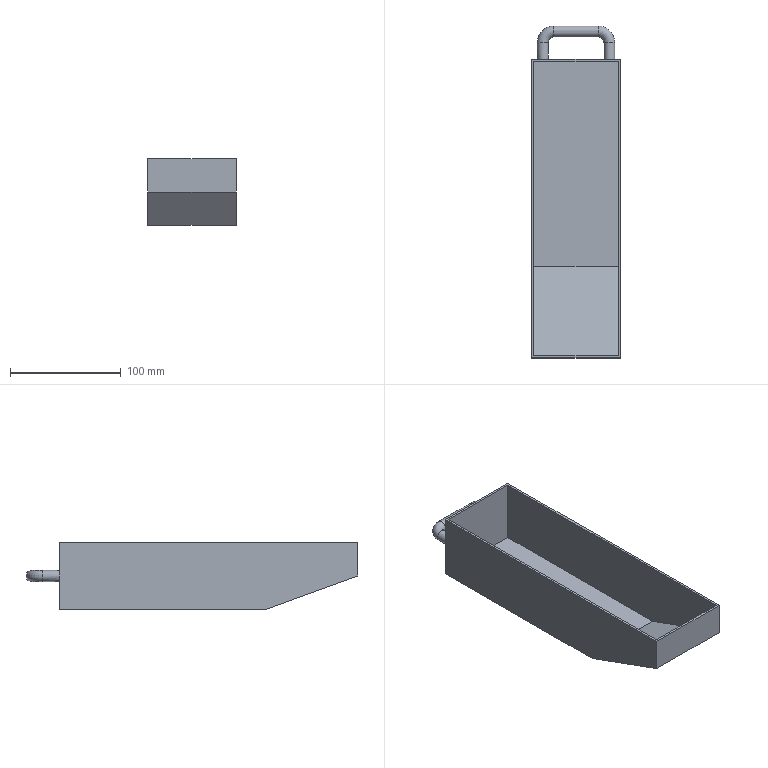Part | NX | features solid 2 | 1 solid | 18 faces | box 80 x 300 x 60 mm | volume 122773 mm3 | plane 13 | cylinder 3 | torus 2 | commonest cylinder face diameters 10 x3
STEP:
#1=CARTESIAN_POINT('',(343.,278.,-283.));
#2=VERTEX_POINT('',#1);
#3=CARTESIAN_POINT('',(343.,92.777,-283.));
#4=VERTEX_POINT('',#3);
#5=CARTESIAN_POINT('',(343.,290.,-283.));
#6=DIRECTION('',(0.,-1.,0.));
#7=VECTOR('',#6,1000.);
#8=LINE('',#5,#7);
#9=EDGE_CURVE('',#2,#4,#8,.T.);
#10=ORIENTED_EDGE('',*,*,#9,.T.);
#11=CARTESIAN_POINT('',(343.,12.,-253.6));
#12=VERTEX_POINT('',#11);
#13=CARTESIAN_POINT('',(343.,274.,-348.96));
#14=DIRECTION('',(0.,-0.9397,0.342));
#15=VECTOR('',#14,1000.);
#16=LINE('',#13,#15);
#17=EDGE_CURVE('',#4,#12,#16,.T.);
#18=ORIENTED_EDGE('',*,*,#17,.T.);
#19=CARTESIAN_POINT('',(343.,12.,-225.));
#20=VERTEX_POINT('',#19);
#21=CARTESIAN_POINT('',(343.,12.,-305.));
#22=DIRECTION('',(0.,0.,1.));
#23=VECTOR('',#22,1000.);
#24=LINE('',#21,#23);
#25=EDGE_CURVE('',#12,#20,#24,.T.);
#26=ORIENTED_EDGE('',*,*,#25,.T.);
#27=CARTESIAN_POINT('',(343.,278.,-225.));
#28=VERTEX_POINT('',#27);
#29=CARTESIAN_POINT('',(343.,290.,-225.));
#30=DIRECTION('',(0.,-1.,0.));
#31=VECTOR('',#30,1000.);
#32=LINE('',#29,#31);
#33=EDGE_CURVE('',#28,#20,#32,.T.);
#34=ORIENTED_EDGE('',*,*,#33,.F.);
#35=CARTESIAN_POINT('',(343.,278.,-305.));
#36=DIRECTION('',(0.,0.,1.));
#37=VECTOR('',#36,1000.);
#38=LINE('',#35,#37);
#39=EDGE_CURVE('',#2,#28,#38,.T.);
#40=ORIENTED_EDGE('',*,*,#39,.F.);
#41=EDGE_LOOP('',(#10,#18,#26,#34,#40));
#42=FACE_BOUND('',#41,.T.);
#43=CARTESIAN_POINT('',(343.,290.,-305.));
#44=DIRECTION('',(-1.,0.,0.));
#45=DIRECTION('',(0.,0.,1.));
#46=AXIS2_PLACEMENT_3D('',#43,#44,#45);
#47=PLANE('',#46);
#48=ADVANCED_FACE('',(#42),#47,.T.);
#49=ORIENTED_EDGE('',*,*,#25,.F.);
#50=CARTESIAN_POINT('',(267.,12.,-253.6));
#51=VERTEX_POINT('',#50);
#52=CARTESIAN_POINT('',(345.,12.,-253.6));
#53=DIRECTION('',(-1.,0.,0.));
#54=VECTOR('',#53,1000.);
#55=LINE('',#52,#54);
#56=EDGE_CURVE('',#12,#51,#55,.T.);
#57=ORIENTED_EDGE('',*,*,#56,.T.);
#58=CARTESIAN_POINT('',(267.,12.,-225.));
#59=VERTEX_POINT('',#58);
#60=CARTESIAN_POINT('',(267.,12.,-305.));
#61=DIRECTION('',(0.,0.,1.));
#62=VECTOR('',#61,1000.);
#63=LINE('',#60,#62);
#64=EDGE_CURVE('',#51,#59,#63,.T.);
#65=ORIENTED_EDGE('',*,*,#64,.T.);
#66=CARTESIAN_POINT('',(345.,12.,-225.));
#67=DIRECTION('',(-1.,0.,0.));
#68=VECTOR('',#67,1000.);
#69=LINE('',#66,#68);
#70=EDGE_CURVE('',#20,#59,#69,.T.);
#71=ORIENTED_EDGE('',*,*,#70,.F.);
#72=EDGE_LOOP('',(#49,#57,#65,#71));
#73=FACE_BOUND('',#72,.T.);
#74=CARTESIAN_POINT('',(345.,12.,-305.));
#75=DIRECTION('',(0.,1.,0.));
#76=DIRECTION('',(0.,0.,1.));
#77=AXIS2_PLACEMENT_3D('',#74,#75,#76);
#78=PLANE('',#77);
#79=ADVANCED_FACE('',(#73),#78,.T.);
#80=ORIENTED_EDGE('',*,*,#64,.F.);
#81=CARTESIAN_POINT('',(267.,92.777,-283.));
#82=VERTEX_POINT('',#81);
#83=CARTESIAN_POINT('',(267.,26.754,-258.97));
#84=DIRECTION('',(0.,0.9397,-0.342));
#85=VECTOR('',#84,1000.);
#86=LINE('',#83,#85);
#87=EDGE_CURVE('',#51,#82,#86,.T.);
#88=ORIENTED_EDGE('',*,*,#87,.T.);
#89=CARTESIAN_POINT('',(267.,278.,-283.));
#90=VERTEX_POINT('',#89);
#91=CARTESIAN_POINT('',(267.,10.,-283.));
#92=DIRECTION('',(0.,1.,0.));
#93=VECTOR('',#92,1000.);
#94=LINE('',#91,#93);
#95=EDGE_CURVE('',#82,#90,#94,.T.);
#96=ORIENTED_EDGE('',*,*,#95,.T.);
#97=CARTESIAN_POINT('',(267.,278.,-225.));
#98=VERTEX_POINT('',#97);
#99=CARTESIAN_POINT('',(267.,278.,-145.));
#100=DIRECTION('',(0.,0.,1.));
#101=VECTOR('',#100,1000.);
#102=LINE('',#99,#101);
#103=EDGE_CURVE('',#90,#98,#102,.T.);
#104=ORIENTED_EDGE('',*,*,#103,.T.);
#105=CARTESIAN_POINT('',(267.,10.,-225.));
#106=DIRECTION('',(0.,1.,0.));
#107=VECTOR('',#106,1000.);
#108=LINE('',#105,#107);
#109=EDGE_CURVE('',#59,#98,#108,.T.);
#110=ORIENTED_EDGE('',*,*,#109,.F.);
#111=EDGE_LOOP('',(#80,#88,#96,#104,#110));
#112=FACE_BOUND('',#111,.T.);
#113=CARTESIAN_POINT('',(267.,10.,-305.));
#114=DIRECTION('',(1.,0.,0.));
#115=DIRECTION('',(0.,0.,-1.));
#116=AXIS2_PLACEMENT_3D('',#113,#114,#115);
#117=PLANE('',#116);
#118=ADVANCED_FACE('',(#112),#117,.T.);
#119=CARTESIAN_POINT('',(345.,92.777,-283.));
#120=DIRECTION('',(-1.,0.,0.));
#121=VECTOR('',#120,1000.);
#122=LINE('',#119,#121);
#123=EDGE_CURVE('',#4,#82,#122,.T.);
#124=ORIENTED_EDGE('',*,*,#123,.F.);
#125=ORIENTED_EDGE('',*,*,#9,.F.);
#126=CARTESIAN_POINT('',(-690.,278.,-283.));
#127=DIRECTION('',(1.,0.,0.));
#128=VECTOR('',#127,1000.);
#129=LINE('',#126,#128);
#130=EDGE_CURVE('',#90,#2,#129,.T.);
#131=ORIENTED_EDGE('',*,*,#130,.F.);
#132=ORIENTED_EDGE('',*,*,#95,.F.);
#133=EDGE_LOOP('',(#124,#125,#131,#132));
#134=FACE_BOUND('',#133,.T.);
#135=CARTESIAN_POINT('',(345.,10.,-283.));
#136=DIRECTION('',(0.,0.,-1.));
#137=DIRECTION('',(-1.,0.,0.));
#138=AXIS2_PLACEMENT_3D('',#135,#136,#137);
#139=PLANE('',#138);
#140=ADVANCED_FACE('',(#134),#139,.F.);
#141=CARTESIAN_POINT('',(335.,280.,-250.));
#142=VERTEX_POINT('',#141);
#143=CARTESIAN_POINT('',(335.,280.,-255.));
#144=DIRECTION('',(0.,-1.,0.));
#145=DIRECTION('',(0.,0.,1.));
#146=AXIS2_PLACEMENT_3D('',#143,#144,#145);
#147=CIRCLE('',#146,5.);
#148=EDGE_CURVE('',#142,#142,#147,.T.);
#149=ORIENTED_EDGE('',*,*,#148,.T.);
#150=EDGE_LOOP('',(#149));
#151=FACE_BOUND('',#150,.T.);
#152=CARTESIAN_POINT('',(265.,280.,-225.));
#153=VERTEX_POINT('',#152);
#154=CARTESIAN_POINT('',(345.,280.,-225.));
#155=VERTEX_POINT('',#154);
#156=CARTESIAN_POINT('',(-690.,280.,-225.));
#157=DIRECTION('',(1.,0.,0.));
#158=VECTOR('',#157,1000.);
#159=LINE('',#156,#158);
#160=EDGE_CURVE('',#153,#155,#159,.T.);
#161=ORIENTED_EDGE('',*,*,#160,.T.);
#162=CARTESIAN_POINT('',(345.,280.,-285.));
#163=VERTEX_POINT('',#162);
#164=CARTESIAN_POINT('',(345.,280.,-305.));
#165=DIRECTION('',(0.,0.,1.));
#166=VECTOR('',#165,1000.);
#167=LINE('',#164,#166);
#168=EDGE_CURVE('',#163,#155,#167,.T.);
#169=ORIENTED_EDGE('',*,*,#168,.F.);
#170=CARTESIAN_POINT('',(265.,280.,-285.));
#171=VERTEX_POINT('',#170);
#172=CARTESIAN_POINT('',(-690.,280.,-285.));
#173=DIRECTION('',(1.,0.,0.));
#174=VECTOR('',#173,1000.);
#175=LINE('',#172,#174);
#176=EDGE_CURVE('',#171,#163,#175,.T.);
#177=ORIENTED_EDGE('',*,*,#176,.F.);
#178=CARTESIAN_POINT('',(265.,280.,-145.));
#179=DIRECTION('',(0.,0.,1.));
#180=VECTOR('',#179,1000.);
#181=LINE('',#178,#180);
#182=EDGE_CURVE('',#171,#153,#181,.T.);
#183=ORIENTED_EDGE('',*,*,#182,.T.);
#184=EDGE_LOOP('',(#161,#169,#177,#183));
#185=FACE_BOUND('',#184,.T.);
#186=CARTESIAN_POINT('',(280.,280.,-255.));
#187=VERTEX_POINT('',#186);
#188=CARTESIAN_POINT('',(275.,280.,-255.));
#189=DIRECTION('',(0.,-1.,0.));
#190=DIRECTION('',(1.,0.,0.));
#191=AXIS2_PLACEMENT_3D('',#188,#189,#190);
#192=CIRCLE('',#191,5.);
#193=EDGE_CURVE('',#187,#187,#192,.F.);
#194=ORIENTED_EDGE('',*,*,#193,.F.);
#195=EDGE_LOOP('',(#194));
#196=FACE_BOUND('',#195,.T.);
#197=CARTESIAN_POINT('',(-690.,280.,-145.));
#198=DIRECTION('',(0.,-1.,0.));
#199=DIRECTION('',(1.,0.,0.));
#200=AXIS2_PLACEMENT_3D('',#197,#198,#199);
#201=PLANE('',#200);
#202=ADVANCED_FACE('',(#151,#185,#196),#201,.F.);
#203=CARTESIAN_POINT('',(345.,10.,-255.));
#204=VERTEX_POINT('',#203);
#205=CARTESIAN_POINT('',(345.,10.,-225.));
#206=VERTEX_POINT('',#205);
#207=CARTESIAN_POINT('',(345.,10.,-305.));
#208=DIRECTION('',(0.,0.,1.));
#209=VECTOR('',#208,1000.);
#210=LINE('',#207,#209);
#211=EDGE_CURVE('',#204,#206,#210,.T.);
#212=ORIENTED_EDGE('',*,*,#211,.F.);
#213=CARTESIAN_POINT('',(345.,92.424,-285.));
#214=VERTEX_POINT('',#213);
#215=CARTESIAN_POINT('',(345.,273.316,-350.839));
#216=DIRECTION('',(0.,0.9397,-0.342));
#217=VECTOR('',#216,1000.);
#218=LINE('',#215,#217);
#219=EDGE_CURVE('',#204,#214,#218,.T.);
#220=ORIENTED_EDGE('',*,*,#219,.T.);
#221=CARTESIAN_POINT('',(345.,290.,-285.));
#222=DIRECTION('',(0.,-1.,0.));
#223=VECTOR('',#222,1000.);
#224=LINE('',#221,#223);
#225=EDGE_CURVE('',#163,#214,#224,.T.);
#226=ORIENTED_EDGE('',*,*,#225,.F.);
#227=ORIENTED_EDGE('',*,*,#168,.T.);
#228=CARTESIAN_POINT('',(345.,290.,-225.));
#229=DIRECTION('',(0.,-1.,0.));
#230=VECTOR('',#229,1000.);
#231=LINE('',#228,#230);
#232=EDGE_CURVE('',#155,#206,#231,.T.);
#233=ORIENTED_EDGE('',*,*,#232,.T.);
#234=EDGE_LOOP('',(#212,#220,#226,#227,#233));
#235=FACE_BOUND('',#234,.T.);
#236=CARTESIAN_POINT('',(345.,290.,-305.));
#237=DIRECTION('',(-1.,0.,0.));
#238=DIRECTION('',(0.,0.,1.));
#239=AXIS2_PLACEMENT_3D('',#236,#237,#238);
#240=PLANE('',#239);
#241=ADVANCED_FACE('',(#235),#240,.F.);
#242=CARTESIAN_POINT('',(265.,10.,-255.));
#243=VERTEX_POINT('',#242);
#244=CARTESIAN_POINT('',(265.,10.,-225.));
#245=VERTEX_POINT('',#244);
#246=CARTESIAN_POINT('',(265.,10.,-305.));
#247=DIRECTION('',(0.,0.,1.));
#248=VECTOR('',#247,1000.);
#249=LINE('',#246,#248);
#250=EDGE_CURVE('',#243,#245,#249,.T.);
#251=ORIENTED_EDGE('',*,*,#250,.F.);
#252=CARTESIAN_POINT('',(345.,10.,-255.));
#253=DIRECTION('',(1.,0.,0.));
#254=VECTOR('',#253,1000.);
#255=LINE('',#252,#254);
#256=EDGE_CURVE('',#243,#204,#255,.T.);
#257=ORIENTED_EDGE('',*,*,#256,.T.);
#258=ORIENTED_EDGE('',*,*,#211,.T.);
#259=CARTESIAN_POINT('',(345.,10.,-225.));
#260=DIRECTION('',(-1.,0.,0.));
#261=VECTOR('',#260,1000.);
#262=LINE('',#259,#261);
#263=EDGE_CURVE('',#206,#245,#262,.T.);
#264=ORIENTED_EDGE('',*,*,#263,.T.);
#265=EDGE_LOOP('',(#251,#257,#258,#264));
#266=FACE_BOUND('',#265,.T.);
#267=CARTESIAN_POINT('',(345.,10.,-305.));
#268=DIRECTION('',(0.,1.,0.));
#269=DIRECTION('',(0.,0.,1.));
#270=AXIS2_PLACEMENT_3D('',#267,#268,#269);
#271=PLANE('',#270);
#272=ADVANCED_FACE('',(#266),#271,.F.);
#273=CARTESIAN_POINT('',(265.,92.424,-285.));
#274=VERTEX_POINT('',#273);
#275=CARTESIAN_POINT('',(265.,10.,-285.));
#276=DIRECTION('',(0.,1.,0.));
#277=VECTOR('',#276,1000.);
#278=LINE('',#275,#277);
#279=EDGE_CURVE('',#274,#171,#278,.T.);
#280=ORIENTED_EDGE('',*,*,#279,.F.);
#281=CARTESIAN_POINT('',(265.,26.07,-260.849));
#282=DIRECTION('',(0.,-0.9397,0.342));
#283=VECTOR('',#282,1000.);
#284=LINE('',#281,#283);
#285=EDGE_CURVE('',#274,#243,#284,.T.);
#286=ORIENTED_EDGE('',*,*,#285,.T.);
#287=ORIENTED_EDGE('',*,*,#250,.T.);
#288=CARTESIAN_POINT('',(265.,10.,-225.));
#289=DIRECTION('',(0.,1.,0.));
#290=VECTOR('',#289,1000.);
#291=LINE('',#288,#290);
#292=EDGE_CURVE('',#245,#153,#291,.T.);
#293=ORIENTED_EDGE('',*,*,#292,.T.);
#294=ORIENTED_EDGE('',*,*,#182,.F.);
#295=EDGE_LOOP('',(#280,#286,#287,#293,#294));
#296=FACE_BOUND('',#295,.T.);
#297=CARTESIAN_POINT('',(265.,10.,-305.));
#298=DIRECTION('',(1.,0.,0.));
#299=DIRECTION('',(0.,0.,-1.));
#300=AXIS2_PLACEMENT_3D('',#297,#298,#299);
#301=PLANE('',#300);
#302=ADVANCED_FACE('',(#296),#301,.F.);
#303=CARTESIAN_POINT('',(345.,92.424,-285.));
#304=DIRECTION('',(1.,0.,0.));
#305=VECTOR('',#304,1000.);
#306=LINE('',#303,#305);
#307=EDGE_CURVE('',#274,#214,#306,.T.);
#308=ORIENTED_EDGE('',*,*,#307,.F.);
#309=ORIENTED_EDGE('',*,*,#279,.T.);
#310=ORIENTED_EDGE('',*,*,#176,.T.);
#311=ORIENTED_EDGE('',*,*,#225,.T.);
#312=EDGE_LOOP('',(#308,#309,#310,#311));
#313=FACE_BOUND('',#312,.T.);
#314=CARTESIAN_POINT('',(345.,10.,-285.));
#315=DIRECTION('',(0.,0.,-1.));
#316=DIRECTION('',(-1.,0.,0.));
#317=AXIS2_PLACEMENT_3D('',#314,#315,#316);
#318=PLANE('',#317);
#319=ADVANCED_FACE('',(#313),#318,.T.);
#320=CARTESIAN_POINT('',(-690.,278.,-225.));
#321=DIRECTION('',(1.,0.,0.));
#322=VECTOR('',#321,1000.);
#323=LINE('',#320,#322);
#324=EDGE_CURVE('',#98,#28,#323,.T.);
#325=ORIENTED_EDGE('',*,*,#324,.T.);
#326=ORIENTED_EDGE('',*,*,#33,.T.);
#327=ORIENTED_EDGE('',*,*,#70,.T.);
#328=ORIENTED_EDGE('',*,*,#109,.T.);
#329=EDGE_LOOP('',(#325,#326,#327,#328));
#330=FACE_BOUND('',#329,.T.);
#331=ORIENTED_EDGE('',*,*,#232,.F.);
#332=ORIENTED_EDGE('',*,*,#160,.F.);
#333=ORIENTED_EDGE('',*,*,#292,.F.);
#334=ORIENTED_EDGE('',*,*,#263,.F.);
#335=EDGE_LOOP('',(#331,#332,#333,#334));
#336=FACE_BOUND('',#335,.T.);
#337=CARTESIAN_POINT('',(345.,10.,-225.));
#338=DIRECTION('',(0.,0.,-1.));
#339=DIRECTION('',(-1.,0.,0.));
#340=AXIS2_PLACEMENT_3D('',#337,#338,#339);
#341=PLANE('',#340);
#342=ADVANCED_FACE('',(#330,#336),#341,.F.);
#343=ORIENTED_EDGE('',*,*,#324,.F.);
#344=ORIENTED_EDGE('',*,*,#103,.F.);
#345=ORIENTED_EDGE('',*,*,#130,.T.);
#346=ORIENTED_EDGE('',*,*,#39,.T.);
#347=EDGE_LOOP('',(#343,#344,#345,#346));
#348=FACE_BOUND('',#347,.T.);
#349=CARTESIAN_POINT('',(-690.,278.,-145.));
#350=DIRECTION('',(0.,-1.,0.));
#351=DIRECTION('',(1.,0.,0.));
#352=AXIS2_PLACEMENT_3D('',#349,#350,#351);
#353=PLANE('',#352);
#354=ADVANCED_FACE('',(#348),#353,.T.);
#355=CARTESIAN_POINT('',(335.,295.,-250.));
#356=VERTEX_POINT('',#355);
#357=CARTESIAN_POINT('',(335.,295.,-255.));
#358=DIRECTION('',(0.,-1.,0.));
#359=DIRECTION('',(0.,0.,1.));
#360=AXIS2_PLACEMENT_3D('',#357,#358,#359);
#361=CIRCLE('',#360,5.);
#362=EDGE_CURVE('',#356,#356,#361,.T.);
#363=ORIENTED_EDGE('',*,*,#362,.T.);
#364=EDGE_LOOP('',(#363));
#365=FACE_BOUND('',#364,.T.);
#366=ORIENTED_EDGE('',*,*,#148,.F.);
#367=EDGE_LOOP('',(#366));
#368=FACE_BOUND('',#367,.T.);
#369=CARTESIAN_POINT('',(335.,295.,-255.));
#370=DIRECTION('',(0.,-1.,0.));
#371=DIRECTION('',(0.,0.,-1.));
#372=AXIS2_PLACEMENT_3D('',#369,#370,#371);
#373=CYLINDRICAL_SURFACE('',#372,5.);
#374=ADVANCED_FACE('',(#365,#368),#373,.T.);
#375=CARTESIAN_POINT('',(325.,305.,-250.));
#376=VERTEX_POINT('',#375);
#377=CARTESIAN_POINT('',(325.,305.,-255.));
#378=DIRECTION('',(1.,0.,0.));
#379=DIRECTION('',(0.,0.,1.));
#380=AXIS2_PLACEMENT_3D('',#377,#378,#379);
#381=CIRCLE('',#380,5.);
#382=EDGE_CURVE('',#376,#376,#381,.T.);
#383=ORIENTED_EDGE('',*,*,#382,.T.);
#384=EDGE_LOOP('',(#383));
#385=FACE_BOUND('',#384,.T.);
#386=ORIENTED_EDGE('',*,*,#362,.F.);
#387=EDGE_LOOP('',(#386));
#388=FACE_BOUND('',#387,.T.);
#389=CARTESIAN_POINT('',(325.,295.,-255.));
#390=DIRECTION('',(0.,0.,-1.));
#391=DIRECTION('',(-1.,0.,0.));
#392=AXIS2_PLACEMENT_3D('',#389,#390,#391);
#393=TOROIDAL_SURFACE('',#392,10.,5.);
#394=ADVANCED_FACE('',(#385,#388),#393,.T.);
#395=CARTESIAN_POINT('',(285.,305.,-250.));
#396=VERTEX_POINT('',#395);
#397=CARTESIAN_POINT('',(285.,305.,-255.));
#398=DIRECTION('',(1.,0.,0.));
#399=DIRECTION('',(0.,0.,1.));
#400=AXIS2_PLACEMENT_3D('',#397,#398,#399);
#401=CIRCLE('',#400,5.);
#402=EDGE_CURVE('',#396,#396,#401,.T.);
#403=ORIENTED_EDGE('',*,*,#402,.T.);
#404=EDGE_LOOP('',(#403));
#405=FACE_BOUND('',#404,.T.);
#406=ORIENTED_EDGE('',*,*,#382,.F.);
#407=EDGE_LOOP('',(#406));
#408=FACE_BOUND('',#407,.T.);
#409=CARTESIAN_POINT('',(285.,305.,-255.));
#410=DIRECTION('',(1.,0.,0.));
#411=DIRECTION('',(0.,0.,-1.));
#412=AXIS2_PLACEMENT_3D('',#409,#410,#411);
#413=CYLINDRICAL_SURFACE('',#412,5.);
#414=ADVANCED_FACE('',(#405,#408),#413,.T.);
#415=CARTESIAN_POINT('',(275.,295.,-250.));
#416=VERTEX_POINT('',#415);
#417=CARTESIAN_POINT('',(275.,295.,-255.));
#418=DIRECTION('',(0.,1.,0.));
#419=DIRECTION('',(0.,0.,1.));
#420=AXIS2_PLACEMENT_3D('',#417,#418,#419);
#421=CIRCLE('',#420,5.);
#422=EDGE_CURVE('',#416,#416,#421,.T.);
#423=ORIENTED_EDGE('',*,*,#422,.T.);
#424=EDGE_LOOP('',(#423));
#425=FACE_BOUND('',#424,.T.);
#426=ORIENTED_EDGE('',*,*,#402,.F.);
#427=EDGE_LOOP('',(#426));
#428=FACE_BOUND('',#427,.T.);
#429=CARTESIAN_POINT('',(285.,295.,-255.));
#430=DIRECTION('',(0.,0.,-1.));
#431=DIRECTION('',(-1.,0.,0.));
#432=AXIS2_PLACEMENT_3D('',#429,#430,#431);
#433=TOROIDAL_SURFACE('',#432,10.,5.);
#434=ADVANCED_FACE('',(#425,#428),#433,.T.);
#435=ORIENTED_EDGE('',*,*,#422,.F.);
#436=EDGE_LOOP('',(#435));
#437=FACE_BOUND('',#436,.T.);
#438=ORIENTED_EDGE('',*,*,#193,.T.);
#439=EDGE_LOOP('',(#438));
#440=FACE_BOUND('',#439,.T.);
#441=CARTESIAN_POINT('',(275.,295.,-255.));
#442=DIRECTION('',(0.,-1.,0.));
#443=DIRECTION('',(0.,0.,-1.));
#444=AXIS2_PLACEMENT_3D('',#441,#442,#443);
#445=CYLINDRICAL_SURFACE('',#444,5.);
#446=ADVANCED_FACE('',(#437,#440),#445,.T.);
#447=ORIENTED_EDGE('',*,*,#219,.F.);
#448=ORIENTED_EDGE('',*,*,#256,.F.);
#449=ORIENTED_EDGE('',*,*,#285,.F.);
#450=ORIENTED_EDGE('',*,*,#307,.T.);
#451=EDGE_LOOP('',(#447,#448,#449,#450));
#452=FACE_BOUND('',#451,.T.);
#453=CARTESIAN_POINT('',(265.,10.,-255.));
#454=DIRECTION('',(0.,0.342,0.9397));
#455=DIRECTION('',(0.,-0.9397,0.342));
#456=AXIS2_PLACEMENT_3D('',#453,#454,#455);
#457=PLANE('',#456);
#458=ADVANCED_FACE('',(#452),#457,.F.);
#459=ORIENTED_EDGE('',*,*,#17,.F.);
#460=ORIENTED_EDGE('',*,*,#123,.T.);
#461=ORIENTED_EDGE('',*,*,#87,.F.);
#462=ORIENTED_EDGE('',*,*,#56,.F.);
#463=EDGE_LOOP('',(#459,#460,#461,#462));
#464=FACE_BOUND('',#463,.T.);
#465=CARTESIAN_POINT('',(365.,93.108,-283.121));
#466=DIRECTION('',(0.,-0.342,-0.9397));
#467=DIRECTION('',(0.,0.9397,-0.342));
#468=AXIS2_PLACEMENT_3D('',#465,#466,#467);
#469=PLANE('',#468);
#470=ADVANCED_FACE('',(#464),#469,.F.);
#471=CLOSED_SHELL('',(#48,#79,#118,#140,#202,#241,#272,#302,#319,#342,#354,#374,#394,#414,#434,#446,#458,#470));
#472=MANIFOLD_SOLID_BREP('',#471);
#473=(LENGTH_UNIT()NAMED_UNIT(*)SI_UNIT(.MILLI.,.METRE.));
#474=UNCERTAINTY_MEASURE_WITH_UNIT(LENGTH_MEASURE(0.00001),#473,'','');
#475=(NAMED_UNIT(*)PLANE_ANGLE_UNIT()SI_UNIT($,.RADIAN.));
#476=(NAMED_UNIT(*)SI_UNIT($,.STERADIAN.)SOLID_ANGLE_UNIT());
#477=(GEOMETRIC_REPRESENTATION_CONTEXT(3)GLOBAL_UNCERTAINTY_ASSIGNED_CONTEXT((#474))GLOBAL_UNIT_ASSIGNED_CONTEXT((#473,#475,#476))REPRESENTATION_CONTEXT('',''));
#478=ADVANCED_BREP_SHAPE_REPRESENTATION('',(#472),#477);